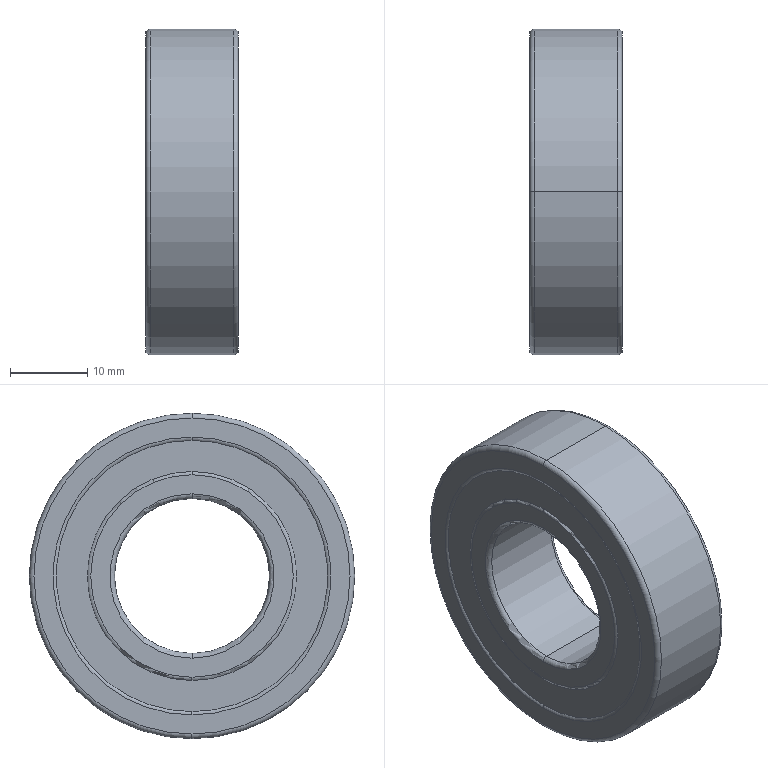Part | STEP file | GB/T 276-2013 deep groove ball bearing 6004-2RZ_6004-2RZ | 16 solids | 188 faces | box 12 x 42 x 42 mm | volume 9713 mm3 | cylinder 66 | sphere 60 | plane 36 | torus 26 | commonest cylinder face diameters 29.9 x27 32.1 x27 27.333 x4 34.667 x4 20 x2 42 x2